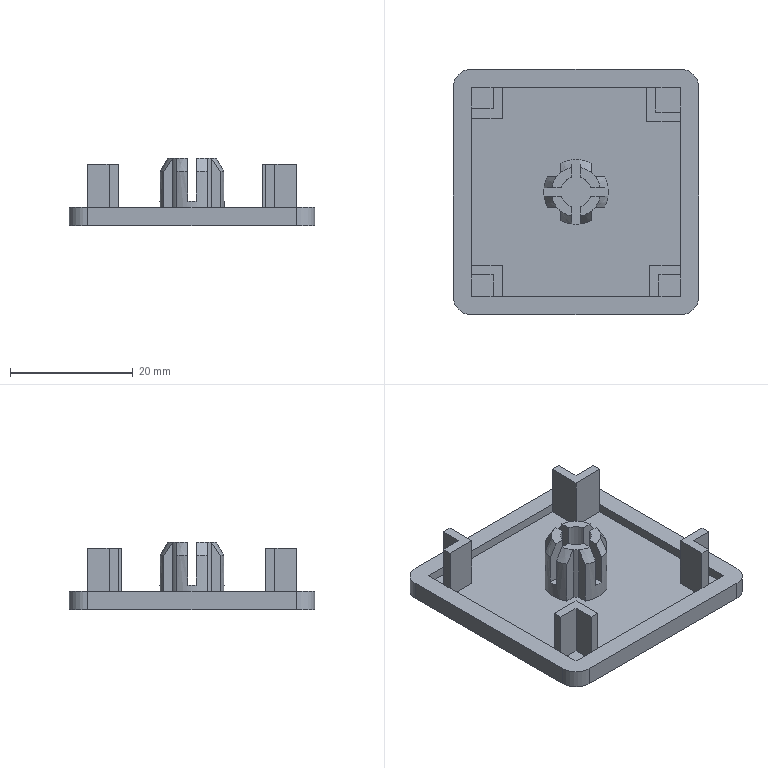Part | SolidWorks | features BaseBody 1 | 1 solid | 97 faces | box 40 x 40 x 11 mm | volume 3954 mm3 | plane 72 | cylinder 17 | cone 8 | commonest cylinder face diameters 10.5 x5 5 x4 6 x4 8 x4